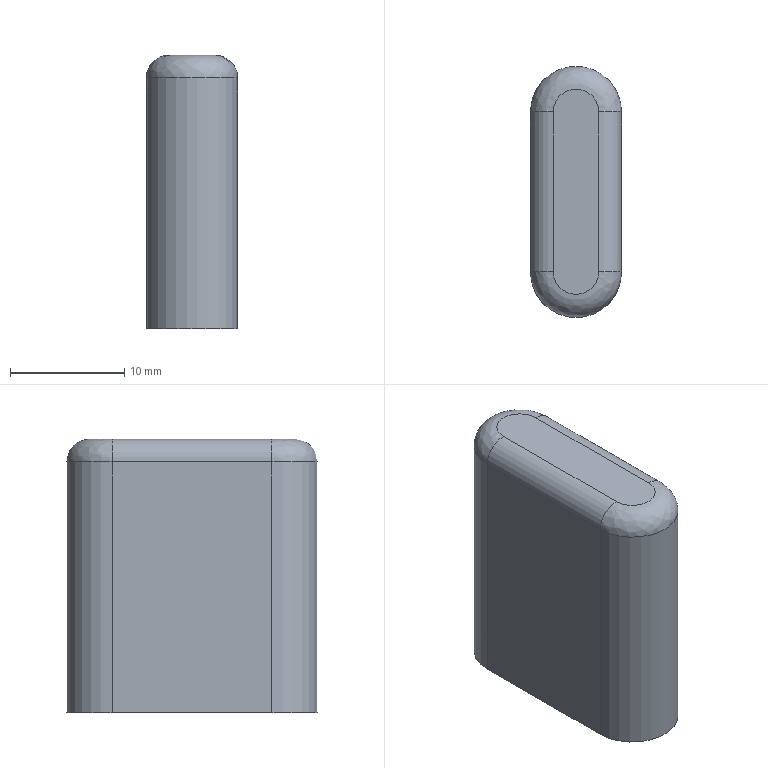Part | STEP file | Tube feed_id510_x_t | 1 solid | 10 faces | box 8 x 22 x 24 mm | volume 3851 mm3 | plane 4 | cylinder 4 | spline 2 | commonest cylinder face diameters 4 x2 8 x2
STEP:
#1=CARTESIAN_POINT('',(0.,0.,0.));
#2=DIRECTION('',(0.,0.,1.));
#3=DIRECTION('',(1.,0.,0.));
#4=AXIS2_PLACEMENT_3D('',#1,#2,#3);
#5=CARTESIAN_POINT('',(380.,467.436,-19.));
#6=VERTEX_POINT('',#5);
#7=CARTESIAN_POINT('',(380.,453.436,-19.));
#8=VERTEX_POINT('',#7);
#9=CARTESIAN_POINT('',(380.,449.436,-19.));
#10=DIRECTION('',(0.,-1.,0.));
#11=VECTOR('',#10,1.);
#12=LINE('',#9,#11);
#13=CARTESIAN_POINT('',(372.,449.436,-19.));
#14=DIRECTION('',(0.,0.,-1.));
#15=DIRECTION('',(0.,1.,0.));
#16=AXIS2_PLACEMENT_3D('',#13,#14,#15);
#17=PLANE('',#16);
#18=CARTESIAN_POINT('',(0.,8.));
#19=DIRECTION('',(-1.,0.));
#20=VECTOR('',#19,1.);
#21=LINE('',#18,#20);
#22=(GEOMETRIC_REPRESENTATION_CONTEXT(2)PARAMETRIC_REPRESENTATION_CONTEXT()REPRESENTATION_CONTEXT('',''));
#23=DEFINITIONAL_REPRESENTATION('',(#21),#22);
#24=PCURVE('',#17,#23);
#25=CARTESIAN_POINT('',(380.,449.436,-18.5));
#26=DIRECTION('',(-1.,0.,0.));
#27=DIRECTION('',(0.,0.,-1.));
#28=AXIS2_PLACEMENT_3D('',#25,#26,#27);
#29=PLANE('',#28);
#30=CARTESIAN_POINT('',(0.5,0.));
#31=DIRECTION('',(0.,1.));
#32=VECTOR('',#31,1.);
#33=LINE('',#30,#32);
#34=(GEOMETRIC_REPRESENTATION_CONTEXT(2)PARAMETRIC_REPRESENTATION_CONTEXT()REPRESENTATION_CONTEXT('',''));
#35=DEFINITIONAL_REPRESENTATION('',(#33),#34);
#36=PCURVE('',#29,#35);
#37=SURFACE_CURVE('',#12,(#24,#36),.PCURVE_S1.);
#38=EDGE_CURVE('',#6,#8,#37,.T.);
#39=ORIENTED_EDGE('',*,*,#38,.T.);
#40=CARTESIAN_POINT('',(372.,453.436,-19.));
#41=VERTEX_POINT('',#40);
#42=CARTESIAN_POINT('',(376.,453.436,-19.));
#43=DIRECTION('',(0.,0.,-1.));
#44=DIRECTION('',(0.,1.,0.));
#45=AXIS2_PLACEMENT_3D('',#42,#43,#44);
#46=CIRCLE('',#45,4.);
#47=CARTESIAN_POINT('',(4.,4.));
#48=DIRECTION('',(1.,0.));
#49=AXIS2_PLACEMENT_2D('',#47,#48);
#50=CIRCLE('',#49,4.);
#51=(GEOMETRIC_REPRESENTATION_CONTEXT(2)PARAMETRIC_REPRESENTATION_CONTEXT()REPRESENTATION_CONTEXT('',''));
#52=DEFINITIONAL_REPRESENTATION('',(#50),#51);
#53=PCURVE('',#17,#52);
#54=CARTESIAN_POINT('',(376.,453.436,-18.5));
#55=DIRECTION('',(0.,0.,-1.));
#56=DIRECTION('',(1.,0.,0.));
#57=AXIS2_PLACEMENT_3D('',#54,#55,#56);
#58=CYLINDRICAL_SURFACE('',#57,4.);
#59=CARTESIAN_POINT('',(-1.571,0.5));
#60=DIRECTION('',(1.,0.));
#61=VECTOR('',#60,1.);
#62=LINE('',#59,#61);
#63=(GEOMETRIC_REPRESENTATION_CONTEXT(2)PARAMETRIC_REPRESENTATION_CONTEXT()REPRESENTATION_CONTEXT('',''));
#64=DEFINITIONAL_REPRESENTATION('',(#62),#63);
#65=PCURVE('',#58,#64);
#66=SURFACE_CURVE('',#46,(#53,#65),.PCURVE_S1.);
#67=EDGE_CURVE('',#8,#41,#66,.T.);
#68=ORIENTED_EDGE('',*,*,#67,.T.);
#69=CARTESIAN_POINT('',(372.,467.436,-19.));
#70=VERTEX_POINT('',#69);
#71=CARTESIAN_POINT('',(372.,449.436,-19.));
#72=DIRECTION('',(0.,-1.,0.));
#73=VECTOR('',#72,1.);
#74=LINE('',#71,#73);
#75=CARTESIAN_POINT('',(0.,0.));
#76=DIRECTION('',(-1.,0.));
#77=VECTOR('',#76,1.);
#78=LINE('',#75,#77);
#79=(GEOMETRIC_REPRESENTATION_CONTEXT(2)PARAMETRIC_REPRESENTATION_CONTEXT()REPRESENTATION_CONTEXT('',''));
#80=DEFINITIONAL_REPRESENTATION('',(#78),#79);
#81=PCURVE('',#17,#80);
#82=CARTESIAN_POINT('',(372.,449.436,-18.5));
#83=DIRECTION('',(-1.,0.,0.));
#84=DIRECTION('',(0.,0.,-1.));
#85=AXIS2_PLACEMENT_3D('',#82,#83,#84);
#86=PLANE('',#85);
#87=CARTESIAN_POINT('',(0.5,0.));
#88=DIRECTION('',(0.,1.));
#89=VECTOR('',#88,1.);
#90=LINE('',#87,#89);
#91=(GEOMETRIC_REPRESENTATION_CONTEXT(2)PARAMETRIC_REPRESENTATION_CONTEXT()REPRESENTATION_CONTEXT('',''));
#92=DEFINITIONAL_REPRESENTATION('',(#90),#91);
#93=PCURVE('',#86,#92);
#94=SURFACE_CURVE('',#74,(#81,#93),.PCURVE_S1.);
#95=EDGE_CURVE('',#70,#41,#94,.T.);
#96=ORIENTED_EDGE('',*,*,#95,.F.);
#97=CARTESIAN_POINT('',(376.,467.436,-19.));
#98=DIRECTION('',(0.,0.,-1.));
#99=DIRECTION('',(0.,1.,0.));
#100=AXIS2_PLACEMENT_3D('',#97,#98,#99);
#101=CIRCLE('',#100,4.);
#102=CARTESIAN_POINT('',(18.,4.));
#103=DIRECTION('',(1.,0.));
#104=AXIS2_PLACEMENT_2D('',#102,#103);
#105=CIRCLE('',#104,4.);
#106=(GEOMETRIC_REPRESENTATION_CONTEXT(2)PARAMETRIC_REPRESENTATION_CONTEXT()REPRESENTATION_CONTEXT('',''));
#107=DEFINITIONAL_REPRESENTATION('',(#105),#106);
#108=PCURVE('',#17,#107);
#109=CARTESIAN_POINT('',(376.,467.436,-18.5));
#110=DIRECTION('',(0.,0.,1.));
#111=DIRECTION('',(-1.,0.,0.));
#112=AXIS2_PLACEMENT_3D('',#109,#110,#111);
#113=CYLINDRICAL_SURFACE('',#112,4.);
#114=CARTESIAN_POINT('',(10.996,-0.5));
#115=DIRECTION('',(-1.,0.));
#116=VECTOR('',#115,1.);
#117=LINE('',#114,#116);
#118=(GEOMETRIC_REPRESENTATION_CONTEXT(2)PARAMETRIC_REPRESENTATION_CONTEXT()REPRESENTATION_CONTEXT('',''));
#119=DEFINITIONAL_REPRESENTATION('',(#117),#118);
#120=PCURVE('',#113,#119);
#121=SURFACE_CURVE('',#101,(#108,#120),.PCURVE_S1.);
#122=EDGE_CURVE('',#70,#6,#121,.T.);
#123=ORIENTED_EDGE('',*,*,#122,.T.);
#124=EDGE_LOOP('',(#39,#68,#96,#123));
#125=FACE_BOUND('',#124,.T.);
#126=ADVANCED_FACE('',(#125),#17,.T.);
#127=CARTESIAN_POINT('',(378.,467.436,5.));
#128=VERTEX_POINT('',#127);
#129=CARTESIAN_POINT('',(374.,467.436,5.));
#130=VERTEX_POINT('',#129);
#131=CARTESIAN_POINT('',(376.,467.436,5.));
#132=DIRECTION('',(0.,0.,1.));
#133=DIRECTION('',(0.,1.,0.));
#134=AXIS2_PLACEMENT_3D('',#131,#132,#133);
#135=CIRCLE('',#134,2.);
#136=CARTESIAN_POINT('',(372.,449.436,5.));
#137=DIRECTION('',(0.,0.,-1.));
#138=DIRECTION('',(0.,1.,0.));
#139=AXIS2_PLACEMENT_3D('',#136,#137,#138);
#140=PLANE('',#139);
#141=CARTESIAN_POINT('',(20.,4.));
#142=CARTESIAN_POINT('',(20.,0.5359));
#143=CARTESIAN_POINT('',(17.,2.268));
#144=CARTESIAN_POINT('',(14.,4.));
#145=CARTESIAN_POINT('',(17.,5.732));
#146=CARTESIAN_POINT('',(20.,7.464));
#147=CARTESIAN_POINT('',(20.,4.));
#148=(BOUNDED_CURVE()B_SPLINE_CURVE(2,(#141,#142,#143,#144,#145,#146,#147),.UNSPECIFIED.,.T.,.F.)B_SPLINE_CURVE_WITH_KNOTS((1,2,2,2,2,1),(-2.094,0.,2.094,4.189,6.283,8.378),.UNSPECIFIED.)CURVE()GEOMETRIC_REPRESENTATION_ITEM()RATIONAL_B_SPLINE_CURVE((1.,0.5,1.,0.5,1.,0.5,1.))REPRESENTATION_ITEM(''));
#149=(GEOMETRIC_REPRESENTATION_CONTEXT(2)PARAMETRIC_REPRESENTATION_CONTEXT()REPRESENTATION_CONTEXT('',''));
#150=DEFINITIONAL_REPRESENTATION('',(#148),#149);
#151=PCURVE('',#140,#150);
#152=CARTESIAN_POINT('',(372.,467.436,3.));
#153=CARTESIAN_POINT('',(372.,475.436,3.));
#154=CARTESIAN_POINT('',(380.,475.436,3.));
#155=CARTESIAN_POINT('',(380.,467.436,3.));
#156=CARTESIAN_POINT('',(372.,467.436,4.172));
#157=CARTESIAN_POINT('',(372.,475.436,4.172));
#158=CARTESIAN_POINT('',(380.,475.436,4.172));
#159=CARTESIAN_POINT('',(380.,467.436,4.172));
#160=CARTESIAN_POINT('',(372.828,467.436,5.));
#161=CARTESIAN_POINT('',(372.828,473.779,5.));
#162=CARTESIAN_POINT('',(379.172,473.779,5.));
#163=CARTESIAN_POINT('',(379.172,467.436,5.));
#164=CARTESIAN_POINT('',(374.,467.436,5.));
#165=CARTESIAN_POINT('',(374.,471.436,5.));
#166=CARTESIAN_POINT('',(378.,471.436,5.));
#167=CARTESIAN_POINT('',(378.,467.436,5.));
#168=(BOUNDED_SURFACE()B_SPLINE_SURFACE(3,3,((#152,#153,#154,#155),(#156,#157,#158,#159),(#160,#161,#162,#163),(#164,#165,#166,#167)),.UNSPECIFIED.,.F.,.F.,.F.)B_SPLINE_SURFACE_WITH_KNOTS((4,4),(4,4),(0.,1.),(0.,1.),.PIECEWISE_BEZIER_KNOTS.)GEOMETRIC_REPRESENTATION_ITEM()RATIONAL_B_SPLINE_SURFACE(((1.,0.3333,0.3333,1.),(0.8047,0.2682,0.2682,0.8047),(0.8047,0.2682,0.2682,0.8047),(1.,0.3333,0.3333,1.)))REPRESENTATION_ITEM('')SURFACE());
#169=CARTESIAN_POINT('',(1.,1.));
#170=CARTESIAN_POINT('',(1.,0.9763));
#171=CARTESIAN_POINT('',(1.,0.9319));
#172=CARTESIAN_POINT('',(1.,0.8733));
#173=CARTESIAN_POINT('',(1.,0.8206));
#174=CARTESIAN_POINT('',(1.,0.7724));
#175=CARTESIAN_POINT('',(1.,0.7279));
#176=CARTESIAN_POINT('',(1.,0.6861));
#177=CARTESIAN_POINT('',(1.,0.6465));
#178=CARTESIAN_POINT('',(1.,0.6086));
#179=CARTESIAN_POINT('',(1.,0.5718));
#180=CARTESIAN_POINT('',(1.,0.5357));
#181=CARTESIAN_POINT('',(1.,0.5));
#182=CARTESIAN_POINT('',(1.,0.4643));
#183=CARTESIAN_POINT('',(1.,0.4282));
#184=CARTESIAN_POINT('',(1.,0.3914));
#185=CARTESIAN_POINT('',(1.,0.3535));
#186=CARTESIAN_POINT('',(1.,0.3139));
#187=CARTESIAN_POINT('',(1.,0.2721));
#188=CARTESIAN_POINT('',(1.,0.2276));
#189=CARTESIAN_POINT('',(1.,0.1794));
#190=CARTESIAN_POINT('',(1.,0.1267));
#191=CARTESIAN_POINT('',(1.,0.06805));
#192=CARTESIAN_POINT('',(1.,0.02375));
#193=CARTESIAN_POINT('',(1.,0.));
#194=B_SPLINE_CURVE_WITH_KNOTS('',3,(#169,#170,#171,#172,#173,#174,#175,#176,#177,#178,#179,#180,#181,#182,#183,#184,#185,#186,#187,#188,#189,#190,#191,#192,#193),.UNSPECIFIED.,.F.,.F.,(4,1,1,1,1,1,1,1,1,1,1,1,1,1,1,1,1,1,1,1,1,1,4),(4.712,4.855,4.998,5.141,5.284,5.426,5.569,5.712,5.855,5.998,6.14,6.283,6.426,6.569,6.712,6.854,6.997,7.14,7.283,7.426,7.568,7.711,7.854),.QUASI_UNIFORM_KNOTS.);
#195=(GEOMETRIC_REPRESENTATION_CONTEXT(2)PARAMETRIC_REPRESENTATION_CONTEXT()REPRESENTATION_CONTEXT('',''));
#196=DEFINITIONAL_REPRESENTATION('',(#194),#195);
#197=PCURVE('',#168,#196);
#198=SURFACE_CURVE('',#135,(#151,#197),.PCURVE_S1.);
#199=EDGE_CURVE('',#128,#130,#198,.T.);
#200=ORIENTED_EDGE('',*,*,#199,.T.);
#201=CARTESIAN_POINT('',(374.,453.436,5.));
#202=VERTEX_POINT('',#201);
#203=CARTESIAN_POINT('',(374.,449.436,5.));
#204=DIRECTION('',(0.,-1.,0.));
#205=VECTOR('',#204,1.);
#206=LINE('',#203,#205);
#207=CARTESIAN_POINT('',(0.,2.));
#208=DIRECTION('',(-1.,0.));
#209=VECTOR('',#208,1.);
#210=LINE('',#207,#209);
#211=(GEOMETRIC_REPRESENTATION_CONTEXT(2)PARAMETRIC_REPRESENTATION_CONTEXT()REPRESENTATION_CONTEXT('',''));
#212=DEFINITIONAL_REPRESENTATION('',(#210),#211);
#213=PCURVE('',#140,#212);
#214=CARTESIAN_POINT('',(374.,449.436,3.));
#215=DIRECTION('',(0.,1.,0.));
#216=DIRECTION('',(0.,0.,1.));
#217=AXIS2_PLACEMENT_3D('',#214,#215,#216);
#218=CYLINDRICAL_SURFACE('',#217,2.);
#219=CARTESIAN_POINT('',(6.283,0.));
#220=DIRECTION('',(0.,-1.));
#221=VECTOR('',#220,1.);
#222=LINE('',#219,#221);
#223=(GEOMETRIC_REPRESENTATION_CONTEXT(2)PARAMETRIC_REPRESENTATION_CONTEXT()REPRESENTATION_CONTEXT('',''));
#224=DEFINITIONAL_REPRESENTATION('',(#222),#223);
#225=PCURVE('',#218,#224);
#226=SURFACE_CURVE('',#206,(#213,#225),.PCURVE_S1.);
#227=EDGE_CURVE('',#130,#202,#226,.T.);
#228=ORIENTED_EDGE('',*,*,#227,.T.);
#229=CARTESIAN_POINT('',(378.,453.436,5.));
#230=VERTEX_POINT('',#229);
#231=CARTESIAN_POINT('',(376.,453.436,5.));
#232=DIRECTION('',(0.,0.,1.));
#233=DIRECTION('',(0.,1.,0.));
#234=AXIS2_PLACEMENT_3D('',#231,#232,#233);
#235=CIRCLE('',#234,2.);
#236=CARTESIAN_POINT('',(6.,4.));
#237=CARTESIAN_POINT('',(6.,0.5359));
#238=CARTESIAN_POINT('',(3.,2.268));
#239=CARTESIAN_POINT('',(0.,4.));
#240=CARTESIAN_POINT('',(3.,5.732));
#241=CARTESIAN_POINT('',(6.,7.464));
#242=CARTESIAN_POINT('',(6.,4.));
#243=(BOUNDED_CURVE()B_SPLINE_CURVE(2,(#236,#237,#238,#239,#240,#241,#242),.UNSPECIFIED.,.T.,.F.)B_SPLINE_CURVE_WITH_KNOTS((1,2,2,2,2,1),(-2.094,0.,2.094,4.189,6.283,8.378),.UNSPECIFIED.)CURVE()GEOMETRIC_REPRESENTATION_ITEM()RATIONAL_B_SPLINE_CURVE((1.,0.5,1.,0.5,1.,0.5,1.))REPRESENTATION_ITEM(''));
#244=(GEOMETRIC_REPRESENTATION_CONTEXT(2)PARAMETRIC_REPRESENTATION_CONTEXT()REPRESENTATION_CONTEXT('',''));
#245=DEFINITIONAL_REPRESENTATION('',(#243),#244);
#246=PCURVE('',#140,#245);
#247=CARTESIAN_POINT('',(380.,453.436,3.));
#248=CARTESIAN_POINT('',(380.,445.436,3.));
#249=CARTESIAN_POINT('',(372.,445.436,3.));
#250=CARTESIAN_POINT('',(372.,453.436,3.));
#251=CARTESIAN_POINT('',(380.,453.436,4.172));
#252=CARTESIAN_POINT('',(380.,445.436,4.172));
#253=CARTESIAN_POINT('',(372.,445.436,4.172));
#254=CARTESIAN_POINT('',(372.,453.436,4.172));
#255=CARTESIAN_POINT('',(379.172,453.436,5.));
#256=CARTESIAN_POINT('',(379.172,447.092,5.));
#257=CARTESIAN_POINT('',(372.828,447.092,5.));
#258=CARTESIAN_POINT('',(372.828,453.436,5.));
#259=CARTESIAN_POINT('',(378.,453.436,5.));
#260=CARTESIAN_POINT('',(378.,449.436,5.));
#261=CARTESIAN_POINT('',(374.,449.436,5.));
#262=CARTESIAN_POINT('',(374.,453.436,5.));
#263=(BOUNDED_SURFACE()B_SPLINE_SURFACE(3,3,((#247,#248,#249,#250),(#251,#252,#253,#254),(#255,#256,#257,#258),(#259,#260,#261,#262)),.UNSPECIFIED.,.F.,.F.,.F.)B_SPLINE_SURFACE_WITH_KNOTS((4,4),(4,4),(0.,1.),(0.,1.),.PIECEWISE_BEZIER_KNOTS.)GEOMETRIC_REPRESENTATION_ITEM()RATIONAL_B_SPLINE_SURFACE(((1.,0.3333,0.3333,1.),(0.8047,0.2682,0.2682,0.8047),(0.8047,0.2682,0.2682,0.8047),(1.,0.3333,0.3333,1.)))REPRESENTATION_ITEM('')SURFACE());
#264=CARTESIAN_POINT('',(1.,1.));
#265=CARTESIAN_POINT('',(1.,0.9763));
#266=CARTESIAN_POINT('',(1.,0.9319));
#267=CARTESIAN_POINT('',(1.,0.8733));
#268=CARTESIAN_POINT('',(1.,0.8206));
#269=CARTESIAN_POINT('',(1.,0.7724));
#270=CARTESIAN_POINT('',(1.,0.7279));
#271=CARTESIAN_POINT('',(1.,0.6861));
#272=CARTESIAN_POINT('',(1.,0.6465));
#273=CARTESIAN_POINT('',(1.,0.6086));
#274=CARTESIAN_POINT('',(1.,0.5718));
#275=CARTESIAN_POINT('',(1.,0.5357));
#276=CARTESIAN_POINT('',(1.,0.5));
#277=CARTESIAN_POINT('',(1.,0.4643));
#278=CARTESIAN_POINT('',(1.,0.4282));
#279=CARTESIAN_POINT('',(1.,0.3914));
#280=CARTESIAN_POINT('',(1.,0.3535));
#281=CARTESIAN_POINT('',(1.,0.3139));
#282=CARTESIAN_POINT('',(1.,0.2721));
#283=CARTESIAN_POINT('',(1.,0.2276));
#284=CARTESIAN_POINT('',(1.,0.1794));
#285=CARTESIAN_POINT('',(1.,0.1267));
#286=CARTESIAN_POINT('',(1.,0.06805));
#287=CARTESIAN_POINT('',(1.,0.02375));
#288=CARTESIAN_POINT('',(1.,0.));
#289=B_SPLINE_CURVE_WITH_KNOTS('',3,(#264,#265,#266,#267,#268,#269,#270,#271,#272,#273,#274,#275,#276,#277,#278,#279,#280,#281,#282,#283,#284,#285,#286,#287,#288),.UNSPECIFIED.,.F.,.F.,(4,1,1,1,1,1,1,1,1,1,1,1,1,1,1,1,1,1,1,1,1,1,4),(1.571,1.714,1.856,1.999,2.142,2.285,2.428,2.57,2.713,2.856,2.999,3.142,3.284,3.427,3.57,3.713,3.856,3.998,4.141,4.284,4.427,4.57,4.712),.QUASI_UNIFORM_KNOTS.);
#290=(GEOMETRIC_REPRESENTATION_CONTEXT(2)PARAMETRIC_REPRESENTATION_CONTEXT()REPRESENTATION_CONTEXT('',''));
#291=DEFINITIONAL_REPRESENTATION('',(#289),#290);
#292=PCURVE('',#263,#291);
#293=SURFACE_CURVE('',#235,(#246,#292),.PCURVE_S1.);
#294=EDGE_CURVE('',#202,#230,#293,.T.);
#295=ORIENTED_EDGE('',*,*,#294,.T.);
#296=CARTESIAN_POINT('',(378.,453.436,5.));
#297=DIRECTION('',(0.,1.,0.));
#298=VECTOR('',#297,1.);
#299=LINE('',#296,#298);
#300=CARTESIAN_POINT('',(4.,6.));
#301=DIRECTION('',(1.,0.));
#302=VECTOR('',#301,1.);
#303=LINE('',#300,#302);
#304=(GEOMETRIC_REPRESENTATION_CONTEXT(2)PARAMETRIC_REPRESENTATION_CONTEXT()REPRESENTATION_CONTEXT('',''));
#305=DEFINITIONAL_REPRESENTATION('',(#303),#304);
#306=PCURVE('',#140,#305);
#307=CARTESIAN_POINT('',(378.,449.436,3.));
#308=DIRECTION('',(0.,-1.,0.));
#309=DIRECTION('',(0.,0.,-1.));
#310=AXIS2_PLACEMENT_3D('',#307,#308,#309);
#311=CYLINDRICAL_SURFACE('',#310,2.);
#312=CARTESIAN_POINT('',(3.142,-4.));
#313=DIRECTION('',(0.,-1.));
#314=VECTOR('',#313,1.);
#315=LINE('',#312,#314);
#316=(GEOMETRIC_REPRESENTATION_CONTEXT(2)PARAMETRIC_REPRESENTATION_CONTEXT()REPRESENTATION_CONTEXT('',''));
#317=DEFINITIONAL_REPRESENTATION('',(#315),#316);
#318=PCURVE('',#311,#317);
#319=SURFACE_CURVE('',#299,(#306,#318),.PCURVE_S1.);
#320=EDGE_CURVE('',#230,#128,#319,.T.);
#321=ORIENTED_EDGE('',*,*,#320,.T.);
#322=EDGE_LOOP('',(#200,#228,#295,#321));
#323=FACE_BOUND('',#322,.T.);
#324=ADVANCED_FACE('',(#323),#140,.F.);
#325=CARTESIAN_POINT('',(380.,453.436,3.));
#326=VERTEX_POINT('',#325);
#327=CARTESIAN_POINT('',(380.,453.436,5.));
#328=DIRECTION('',(0.,0.,-1.));
#329=VECTOR('',#328,1.);
#330=LINE('',#327,#329);
#331=CARTESIAN_POINT('',(-23.5,-4.));
#332=DIRECTION('',(1.,0.));
#333=VECTOR('',#332,1.);
#334=LINE('',#331,#333);
#335=(GEOMETRIC_REPRESENTATION_CONTEXT(2)PARAMETRIC_REPRESENTATION_CONTEXT()REPRESENTATION_CONTEXT('',''));
#336=DEFINITIONAL_REPRESENTATION('',(#334),#335);
#337=PCURVE('',#29,#336);
#338=CARTESIAN_POINT('',(0.,-23.5));
#339=DIRECTION('',(0.,1.));
#340=VECTOR('',#339,1.);
#341=LINE('',#338,#340);
#342=(GEOMETRIC_REPRESENTATION_CONTEXT(2)PARAMETRIC_REPRESENTATION_CONTEXT()REPRESENTATION_CONTEXT('',''));
#343=DEFINITIONAL_REPRESENTATION('',(#341),#342);
#344=PCURVE('',#58,#343);
#345=SURFACE_CURVE('',#330,(#337,#344),.PCURVE_S1.);
#346=EDGE_CURVE('',#326,#8,#345,.T.);
#347=ORIENTED_EDGE('',*,*,#346,.T.);
#348=ORIENTED_EDGE('',*,*,#38,.F.);
#349=CARTESIAN_POINT('',(380.,467.436,3.));
#350=VERTEX_POINT('',#349);
#351=CARTESIAN_POINT('',(380.,467.436,-18.5));
#352=DIRECTION('',(0.,0.,1.));
#353=VECTOR('',#352,1.);
#354=LINE('',#351,#353);
#355=CARTESIAN_POINT('',(0.,-18.));
#356=DIRECTION('',(-1.,0.));
#357=VECTOR('',#356,1.);
#358=LINE('',#355,#357);
#359=(GEOMETRIC_REPRESENTATION_CONTEXT(2)PARAMETRIC_REPRESENTATION_CONTEXT()REPRESENTATION_CONTEXT('',''));
#360=DEFINITIONAL_REPRESENTATION('',(#358),#359);
#361=PCURVE('',#29,#360);
#362=CARTESIAN_POINT('',(3.142,0.));
#363=DIRECTION('',(0.,1.));
#364=VECTOR('',#363,1.);
#365=LINE('',#362,#364);
#366=(GEOMETRIC_REPRESENTATION_CONTEXT(2)PARAMETRIC_REPRESENTATION_CONTEXT()REPRESENTATION_CONTEXT('',''));
#367=DEFINITIONAL_REPRESENTATION('',(#365),#366);
#368=PCURVE('',#113,#367);
#369=SURFACE_CURVE('',#354,(#361,#368),.PCURVE_S1.);
#370=EDGE_CURVE('',#6,#350,#369,.T.);
#371=ORIENTED_EDGE('',*,*,#370,.T.);
#372=CARTESIAN_POINT('',(380.,467.436,3.));
#373=DIRECTION('',(0.,-1.,0.));
#374=VECTOR('',#373,1.);
#375=LINE('',#372,#374);
#376=CARTESIAN_POINT('',(-21.5,-18.));
#377=DIRECTION('',(0.,1.));
#378=VECTOR('',#377,1.);
#379=LINE('',#376,#378);
#380=(GEOMETRIC_REPRESENTATION_CONTEXT(2)PARAMETRIC_REPRESENTATION_CONTEXT()REPRESENTATION_CONTEXT('',''));
#381=DEFINITIONAL_REPRESENTATION('',(#379),#380);
#382=PCURVE('',#29,#381);
#383=CARTESIAN_POINT('',(1.571,-18.));
#384=DIRECTION('',(0.,1.));
#385=VECTOR('',#384,1.);
#386=LINE('',#383,#385);
#387=(GEOMETRIC_REPRESENTATION_CONTEXT(2)PARAMETRIC_REPRESENTATION_CONTEXT()REPRESENTATION_CONTEXT('',''));
#388=DEFINITIONAL_REPRESENTATION('',(#386),#387);
#389=PCURVE('',#311,#388);
#390=SURFACE_CURVE('',#375,(#382,#389),.PCURVE_S1.);
#391=EDGE_CURVE('',#350,#326,#390,.T.);
#392=ORIENTED_EDGE('',*,*,#391,.T.);
#393=EDGE_LOOP('',(#347,#348,#371,#392));
#394=FACE_BOUND('',#393,.T.);
#395=ADVANCED_FACE('',(#394),#29,.F.);
#396=CARTESIAN_POINT('',(372.,467.436,3.));
#397=VERTEX_POINT('',#396);
#398=CARTESIAN_POINT('',(372.,467.436,-18.5));
#399=DIRECTION('',(0.,0.,-1.));
#400=VECTOR('',#399,1.);
#401=LINE('',#398,#400);
#402=CARTESIAN_POINT('',(0.,-18.));
#403=DIRECTION('',(1.,0.));
#404=VECTOR('',#403,1.);
#405=LINE('',#402,#404);
#406=(GEOMETRIC_REPRESENTATION_CONTEXT(2)PARAMETRIC_REPRESENTATION_CONTEXT()REPRESENTATION_CONTEXT('',''));
#407=DEFINITIONAL_REPRESENTATION('',(#405),#406);
#408=PCURVE('',#86,#407);
#409=CARTESIAN_POINT('',(6.283,0.));
#410=DIRECTION('',(0.,-1.));
#411=VECTOR('',#410,1.);
#412=LINE('',#409,#411);
#413=(GEOMETRIC_REPRESENTATION_CONTEXT(2)PARAMETRIC_REPRESENTATION_CONTEXT()REPRESENTATION_CONTEXT('',''));
#414=DEFINITIONAL_REPRESENTATION('',(#412),#413);
#415=PCURVE('',#113,#414);
#416=SURFACE_CURVE('',#401,(#408,#415),.PCURVE_S1.);
#417=EDGE_CURVE('',#397,#70,#416,.T.);
#418=ORIENTED_EDGE('',*,*,#417,.T.);
#419=ORIENTED_EDGE('',*,*,#95,.T.);
#420=CARTESIAN_POINT('',(372.,453.436,3.));
#421=VERTEX_POINT('',#420);
#422=CARTESIAN_POINT('',(372.,453.436,-18.5));
#423=DIRECTION('',(0.,0.,1.));
#424=VECTOR('',#423,1.);
#425=LINE('',#422,#424);
#426=CARTESIAN_POINT('',(0.,-4.));
#427=DIRECTION('',(-1.,0.));
#428=VECTOR('',#427,1.);
#429=LINE('',#426,#428);
#430=(GEOMETRIC_REPRESENTATION_CONTEXT(2)PARAMETRIC_REPRESENTATION_CONTEXT()REPRESENTATION_CONTEXT('',''));
#431=DEFINITIONAL_REPRESENTATION('',(#429),#430);
#432=PCURVE('',#86,#431);
#433=CARTESIAN_POINT('',(3.142,0.));
#434=DIRECTION('',(0.,-1.));
#435=VECTOR('',#434,1.);
#436=LINE('',#433,#435);
#437=(GEOMETRIC_REPRESENTATION_CONTEXT(2)PARAMETRIC_REPRESENTATION_CONTEXT()REPRESENTATION_CONTEXT('',''));
#438=DEFINITIONAL_REPRESENTATION('',(#436),#437);
#439=PCURVE('',#58,#438);
#440=SURFACE_CURVE('',#425,(#432,#439),.PCURVE_S1.);
#441=EDGE_CURVE('',#41,#421,#440,.T.);
#442=ORIENTED_EDGE('',*,*,#441,.T.);
#443=CARTESIAN_POINT('',(372.,449.436,3.));
#444=DIRECTION('',(0.,1.,0.));
#445=VECTOR('',#444,1.);
#446=LINE('',#443,#445);
#447=CARTESIAN_POINT('',(-21.5,0.));
#448=DIRECTION('',(0.,-1.));
#449=VECTOR('',#448,1.);
#450=LINE('',#447,#449);
#451=(GEOMETRIC_REPRESENTATION_CONTEXT(2)PARAMETRIC_REPRESENTATION_CONTEXT()REPRESENTATION_CONTEXT('',''));
#452=DEFINITIONAL_REPRESENTATION('',(#450),#451);
#453=PCURVE('',#86,#452);
#454=CARTESIAN_POINT('',(4.712,0.));
#455=DIRECTION('',(0.,1.));
#456=VECTOR('',#455,1.);
#457=LINE('',#454,#456);
#458=(GEOMETRIC_REPRESENTATION_CONTEXT(2)PARAMETRIC_REPRESENTATION_CONTEXT()REPRESENTATION_CONTEXT('',''));
#459=DEFINITIONAL_REPRESENTATION('',(#457),#458);
#460=PCURVE('',#218,#459);
#461=SURFACE_CURVE('',#446,(#453,#460),.PCURVE_S1.);
#462=EDGE_CURVE('',#421,#397,#461,.T.);
#463=ORIENTED_EDGE('',*,*,#462,.T.);
#464=EDGE_LOOP('',(#418,#419,#442,#463));
#465=FACE_BOUND('',#464,.T.);
#466=ADVANCED_FACE('',(#465),#86,.T.);
#467=ORIENTED_EDGE('',*,*,#370,.F.);
#468=ORIENTED_EDGE('',*,*,#122,.F.);
#469=ORIENTED_EDGE('',*,*,#417,.F.);
#470=CARTESIAN_POINT('',(376.,467.436,3.));
#471=DIRECTION('',(0.,0.,-1.));
#472=DIRECTION('',(0.,1.,0.));
#473=AXIS2_PLACEMENT_3D('',#470,#471,#472);
#474=CIRCLE('',#473,4.);
#475=CARTESIAN_POINT('',(10.996,21.5));
#476=DIRECTION('',(-1.,0.));
#477=VECTOR('',#476,1.);
#478=LINE('',#475,#477);
#479=(GEOMETRIC_REPRESENTATION_CONTEXT(2)PARAMETRIC_REPRESENTATION_CONTEXT()REPRESENTATION_CONTEXT('',''));
#480=DEFINITIONAL_REPRESENTATION('',(#478),#479);
#481=PCURVE('',#113,#480);
#482=CARTESIAN_POINT('',(0.,0.));
#483=CARTESIAN_POINT('',(0.,0.02375));
#484=CARTESIAN_POINT('',(0.,0.06805));
#485=CARTESIAN_POINT('',(0.,0.1267));
#486=CARTESIAN_POINT('',(0.,0.1794));
#487=CARTESIAN_POINT('',(0.,0.2276));
#488=CARTESIAN_POINT('',(0.,0.2721));
#489=CARTESIAN_POINT('',(0.,0.3139));
#490=CARTESIAN_POINT('',(0.,0.3535));
#491=CARTESIAN_POINT('',(0.,0.3914));
#492=CARTESIAN_POINT('',(0.,0.4282));
#493=CARTESIAN_POINT('',(0.,0.4643));
#494=CARTESIAN_POINT('',(0.,0.5));
#495=CARTESIAN_POINT('',(0.,0.5357));
#496=CARTESIAN_POINT('',(0.,0.5718));
#497=CARTESIAN_POINT('',(0.,0.6086));
#498=CARTESIAN_POINT('',(0.,0.6465));
#499=CARTESIAN_POINT('',(0.,0.6861));
#500=CARTESIAN_POINT('',(0.,0.7279));
#501=CARTESIAN_POINT('',(0.,0.7724));
#502=CARTESIAN_POINT('',(0.,0.8206));
#503=CARTESIAN_POINT('',(0.,0.8733));
#504=CARTESIAN_POINT('',(0.,0.9319));
#505=CARTESIAN_POINT('',(0.,0.9763));
#506=CARTESIAN_POINT('',(0.,1.));
#507=B_SPLINE_CURVE_WITH_KNOTS('',3,(#482,#483,#484,#485,#486,#487,#488,#489,#490,#491,#492,#493,#494,#495,#496,#497,#498,#499,#500,#501,#502,#503,#504,#505,#506),.UNSPECIFIED.,.F.,.F.,(4,1,1,1,1,1,1,1,1,1,1,1,1,1,1,1,1,1,1,1,1,1,4),(4.712,4.855,4.998,5.141,5.284,5.426,5.569,5.712,5.855,5.998,6.14,6.283,6.426,6.569,6.712,6.854,6.997,7.14,7.283,7.426,7.568,7.711,7.854),.QUASI_UNIFORM_KNOTS.);
#508=(GEOMETRIC_REPRESENTATION_CONTEXT(2)PARAMETRIC_REPRESENTATION_CONTEXT()REPRESENTATION_CONTEXT('',''));
#509=DEFINITIONAL_REPRESENTATION('',(#507),#508);
#510=PCURVE('',#168,#509);
#511=SURFACE_CURVE('',#474,(#481,#510),.PCURVE_S1.);
#512=EDGE_CURVE('',#397,#350,#511,.T.);
#513=ORIENTED_EDGE('',*,*,#512,.T.);
#514=EDGE_LOOP('',(#467,#468,#469,#513));
#515=FACE_BOUND('',#514,.T.);
#516=ADVANCED_FACE('',(#515),#113,.T.);
#517=ORIENTED_EDGE('',*,*,#441,.F.);
#518=ORIENTED_EDGE('',*,*,#67,.F.);
#519=ORIENTED_EDGE('',*,*,#346,.F.);
#520=CARTESIAN_POINT('',(376.,453.436,3.));
#521=DIRECTION('',(0.,0.,-1.));
#522=DIRECTION('',(0.,1.,0.));
#523=AXIS2_PLACEMENT_3D('',#520,#521,#522);
#524=CIRCLE('',#523,4.);
#525=CARTESIAN_POINT('',(-1.571,-21.5));
#526=DIRECTION('',(1.,0.));
#527=VECTOR('',#526,1.);
#528=LINE('',#525,#527);
#529=(GEOMETRIC_REPRESENTATION_CONTEXT(2)PARAMETRIC_REPRESENTATION_CONTEXT()REPRESENTATION_CONTEXT('',''));
#530=DEFINITIONAL_REPRESENTATION('',(#528),#529);
#531=PCURVE('',#58,#530);
#532=CARTESIAN_POINT('',(0.,0.));
#533=CARTESIAN_POINT('',(0.,0.02375));
#534=CARTESIAN_POINT('',(0.,0.06805));
#535=CARTESIAN_POINT('',(0.,0.1267));
#536=CARTESIAN_POINT('',(0.,0.1794));
#537=CARTESIAN_POINT('',(0.,0.2276));
#538=CARTESIAN_POINT('',(0.,0.2721));
#539=CARTESIAN_POINT('',(0.,0.3139));
#540=CARTESIAN_POINT('',(0.,0.3535));
#541=CARTESIAN_POINT('',(0.,0.3914));
#542=CARTESIAN_POINT('',(0.,0.4282));
#543=CARTESIAN_POINT('',(0.,0.4643));
#544=CARTESIAN_POINT('',(0.,0.5));
#545=CARTESIAN_POINT('',(0.,0.5357));
#546=CARTESIAN_POINT('',(0.,0.5718));
#547=CARTESIAN_POINT('',(0.,0.6086));
#548=CARTESIAN_POINT('',(0.,0.6465));
#549=CARTESIAN_POINT('',(0.,0.6861));
#550=CARTESIAN_POINT('',(0.,0.7279));
#551=CARTESIAN_POINT('',(0.,0.7724));
#552=CARTESIAN_POINT('',(0.,0.8206));
#553=CARTESIAN_POINT('',(0.,0.8733));
#554=CARTESIAN_POINT('',(0.,0.9319));
#555=CARTESIAN_POINT('',(0.,0.9763));
#556=CARTESIAN_POINT('',(0.,1.));
#557=B_SPLINE_CURVE_WITH_KNOTS('',3,(#532,#533,#534,#535,#536,#537,#538,#539,#540,#541,#542,#543,#544,#545,#546,#547,#548,#549,#550,#551,#552,#553,#554,#555,#556),.UNSPECIFIED.,.F.,.F.,(4,1,1,1,1,1,1,1,1,1,1,1,1,1,1,1,1,1,1,1,1,1,4),(1.571,1.714,1.856,1.999,2.142,2.285,2.428,2.57,2.713,2.856,2.999,3.142,3.284,3.427,3.57,3.713,3.856,3.998,4.141,4.284,4.427,4.57,4.712),.QUASI_UNIFORM_KNOTS.);
#558=(GEOMETRIC_REPRESENTATION_CONTEXT(2)PARAMETRIC_REPRESENTATION_CONTEXT()REPRESENTATION_CONTEXT('',''));
#559=DEFINITIONAL_REPRESENTATION('',(#557),#558);
#560=PCURVE('',#263,#559);
#561=SURFACE_CURVE('',#524,(#531,#560),.PCURVE_S1.);
#562=EDGE_CURVE('',#326,#421,#561,.T.);
#563=ORIENTED_EDGE('',*,*,#562,.T.);
#564=EDGE_LOOP('',(#517,#518,#519,#563));
#565=FACE_BOUND('',#564,.T.);
#566=ADVANCED_FACE('',(#565),#58,.T.);
#567=CARTESIAN_POINT('',(374.,453.436,3.));
#568=DIRECTION('',(0.,-1.,0.));
#569=DIRECTION('',(0.,0.,-1.));
#570=AXIS2_PLACEMENT_3D('',#567,#568,#569);
#571=CIRCLE('',#570,2.);
#572=CARTESIAN_POINT('',(9.425,4.));
#573=DIRECTION('',(-1.,0.));
#574=VECTOR('',#573,1.);
#575=LINE('',#572,#574);
#576=(GEOMETRIC_REPRESENTATION_CONTEXT(2)PARAMETRIC_REPRESENTATION_CONTEXT()REPRESENTATION_CONTEXT('',''));
#577=DEFINITIONAL_REPRESENTATION('',(#575),#576);
#578=PCURVE('',#218,#577);
#579=CARTESIAN_POINT('',(1.,1.));
#580=CARTESIAN_POINT('',(0.9832,1.));
#581=CARTESIAN_POINT('',(0.95,1.));
#582=CARTESIAN_POINT('',(0.9016,1.));
#583=CARTESIAN_POINT('',(0.8543,1.));
#584=CARTESIAN_POINT('',(0.808,1.));
#585=CARTESIAN_POINT('',(0.7625,1.));
#586=CARTESIAN_POINT('',(0.7177,1.));
#587=CARTESIAN_POINT('',(0.6735,1.));
#588=CARTESIAN_POINT('',(0.6297,1.));
#589=CARTESIAN_POINT('',(0.5863,1.));
#590=CARTESIAN_POINT('',(0.5431,1.));
#591=CARTESIAN_POINT('',(0.5,1.));
#592=CARTESIAN_POINT('',(0.4569,1.));
#593=CARTESIAN_POINT('',(0.4137,1.));
#594=CARTESIAN_POINT('',(0.3703,1.));
#595=CARTESIAN_POINT('',(0.3265,1.));
#596=CARTESIAN_POINT('',(0.2823,1.));
#597=CARTESIAN_POINT('',(0.2375,1.));
#598=CARTESIAN_POINT('',(0.192,1.));
#599=CARTESIAN_POINT('',(0.1457,1.));
#600=CARTESIAN_POINT('',(0.09843,1.));
#601=CARTESIAN_POINT('',(0.04999,1.));
#602=CARTESIAN_POINT('',(0.01683,1.));
#603=CARTESIAN_POINT('',(0.,1.));
#604=B_SPLINE_CURVE_WITH_KNOTS('',3,(#579,#580,#581,#582,#583,#584,#585,#586,#587,#588,#589,#590,#591,#592,#593,#594,#595,#596,#597,#598,#599,#600,#601,#602,#603),.UNSPECIFIED.,.F.,.F.,(4,1,1,1,1,1,1,1,1,1,1,1,1,1,1,1,1,1,1,1,1,1,4),(3.142,3.213,3.284,3.356,3.427,3.499,3.57,3.641,3.713,3.784,3.856,3.927,3.998,4.07,4.141,4.213,4.284,4.355,4.427,4.498,4.57,4.641,4.712),.QUASI_UNIFORM_KNOTS.);
#605=(GEOMETRIC_REPRESENTATION_CONTEXT(2)PARAMETRIC_REPRESENTATION_CONTEXT()REPRESENTATION_CONTEXT('',''));
#606=DEFINITIONAL_REPRESENTATION('',(#604),#605);
#607=PCURVE('',#263,#606);
#608=SURFACE_CURVE('',#571,(#578,#607),.PCURVE_S1.);
#609=EDGE_CURVE('',#202,#421,#608,.T.);
#610=ORIENTED_EDGE('',*,*,#609,.F.);
#611=ORIENTED_EDGE('',*,*,#227,.F.);
#612=CARTESIAN_POINT('',(374.,467.436,3.));
#613=DIRECTION('',(0.,1.,0.));
#614=DIRECTION('',(0.,0.,1.));
#615=AXIS2_PLACEMENT_3D('',#612,#613,#614);
#616=CIRCLE('',#615,2.);
#617=CARTESIAN_POINT('',(0.,18.));
#618=DIRECTION('',(1.,0.));
#619=VECTOR('',#618,1.);
#620=LINE('',#617,#619);
#621=(GEOMETRIC_REPRESENTATION_CONTEXT(2)PARAMETRIC_REPRESENTATION_CONTEXT()REPRESENTATION_CONTEXT('',''));
#622=DEFINITIONAL_REPRESENTATION('',(#620),#621);
#623=PCURVE('',#218,#622);
#624=CARTESIAN_POINT('',(0.,0.));
#625=CARTESIAN_POINT('',(0.01683,0.));
#626=CARTESIAN_POINT('',(0.04999,0.));
#627=CARTESIAN_POINT('',(0.09843,0.));
#628=CARTESIAN_POINT('',(0.1457,0.));
#629=CARTESIAN_POINT('',(0.192,0.));
#630=CARTESIAN_POINT('',(0.2375,0.));
#631=CARTESIAN_POINT('',(0.2823,0.));
#632=CARTESIAN_POINT('',(0.3265,0.));
#633=CARTESIAN_POINT('',(0.3703,0.));
#634=CARTESIAN_POINT('',(0.4137,0.));
#635=CARTESIAN_POINT('',(0.4569,0.));
#636=CARTESIAN_POINT('',(0.5,0.));
#637=CARTESIAN_POINT('',(0.5431,0.));
#638=CARTESIAN_POINT('',(0.5863,0.));
#639=CARTESIAN_POINT('',(0.6297,0.));
#640=CARTESIAN_POINT('',(0.6735,0.));
#641=CARTESIAN_POINT('',(0.7177,0.));
#642=CARTESIAN_POINT('',(0.7625,0.));
#643=CARTESIAN_POINT('',(0.808,0.));
#644=CARTESIAN_POINT('',(0.8543,0.));
#645=CARTESIAN_POINT('',(0.9016,0.));
#646=CARTESIAN_POINT('',(0.95,0.));
#647=CARTESIAN_POINT('',(0.9832,0.));
#648=CARTESIAN_POINT('',(1.,0.));
#649=B_SPLINE_CURVE_WITH_KNOTS('',3,(#624,#625,#626,#627,#628,#629,#630,#631,#632,#633,#634,#635,#636,#637,#638,#639,#640,#641,#642,#643,#644,#645,#646,#647,#648),.UNSPECIFIED.,.F.,.F.,(4,1,1,1,1,1,1,1,1,1,1,1,1,1,1,1,1,1,1,1,1,1,4),(4.712,4.784,4.855,4.927,4.998,5.069,5.141,5.212,5.284,5.355,5.426,5.498,5.569,5.641,5.712,5.783,5.855,5.926,5.998,6.069,6.14,6.212,6.283),.QUASI_UNIFORM_KNOTS.);
#650=(GEOMETRIC_REPRESENTATION_CONTEXT(2)PARAMETRIC_REPRESENTATION_CONTEXT()REPRESENTATION_CONTEXT('',''));
#651=DEFINITIONAL_REPRESENTATION('',(#649),#650);
#652=PCURVE('',#168,#651);
#653=SURFACE_CURVE('',#616,(#623,#652),.PCURVE_S1.);
#654=EDGE_CURVE('',#397,#130,#653,.T.);
#655=ORIENTED_EDGE('',*,*,#654,.F.);
#656=ORIENTED_EDGE('',*,*,#462,.F.);
#657=EDGE_LOOP('',(#610,#611,#655,#656));
#658=FACE_BOUND('',#657,.T.);
#659=ADVANCED_FACE('',(#658),#218,.T.);
#660=ORIENTED_EDGE('',*,*,#654,.T.);
#661=ORIENTED_EDGE('',*,*,#199,.F.);
#662=CARTESIAN_POINT('',(378.,467.436,3.));
#663=DIRECTION('',(0.,-1.,0.));
#664=DIRECTION('',(0.,0.,-1.));
#665=AXIS2_PLACEMENT_3D('',#662,#663,#664);
#666=CIRCLE('',#665,2.);
#667=CARTESIAN_POINT('',(0.,1.));
#668=CARTESIAN_POINT('',(0.01683,1.));
#669=CARTESIAN_POINT('',(0.04999,1.));
#670=CARTESIAN_POINT('',(0.09843,1.));
#671=CARTESIAN_POINT('',(0.1457,1.));
#672=CARTESIAN_POINT('',(0.192,1.));
#673=CARTESIAN_POINT('',(0.2375,1.));
#674=CARTESIAN_POINT('',(0.2823,1.));
#675=CARTESIAN_POINT('',(0.3265,1.));
#676=CARTESIAN_POINT('',(0.3703,1.));
#677=CARTESIAN_POINT('',(0.4137,1.));
#678=CARTESIAN_POINT('',(0.4569,1.));
#679=CARTESIAN_POINT('',(0.5,1.));
#680=CARTESIAN_POINT('',(0.5431,1.));
#681=CARTESIAN_POINT('',(0.5863,1.));
#682=CARTESIAN_POINT('',(0.6297,1.));
#683=CARTESIAN_POINT('',(0.6735,1.));
#684=CARTESIAN_POINT('',(0.7177,1.));
#685=CARTESIAN_POINT('',(0.7625,1.));
#686=CARTESIAN_POINT('',(0.808,1.));
#687=CARTESIAN_POINT('',(0.8543,1.));
#688=CARTESIAN_POINT('',(0.9016,1.));
#689=CARTESIAN_POINT('',(0.95,1.));
#690=CARTESIAN_POINT('',(0.9832,1.));
#691=CARTESIAN_POINT('',(1.,1.));
#692=B_SPLINE_CURVE_WITH_KNOTS('',3,(#667,#668,#669,#670,#671,#672,#673,#674,#675,#676,#677,#678,#679,#680,#681,#682,#683,#684,#685,#686,#687,#688,#689,#690,#691),.UNSPECIFIED.,.F.,.F.,(4,1,1,1,1,1,1,1,1,1,1,1,1,1,1,1,1,1,1,1,1,1,4),(1.571,1.642,1.714,1.785,1.856,1.928,1.999,2.071,2.142,2.213,2.285,2.356,2.428,2.499,2.57,2.642,2.713,2.785,2.856,2.927,2.999,3.07,3.142),.QUASI_UNIFORM_KNOTS.);
#693=(GEOMETRIC_REPRESENTATION_CONTEXT(2)PARAMETRIC_REPRESENTATION_CONTEXT()REPRESENTATION_CONTEXT('',''));
#694=DEFINITIONAL_REPRESENTATION('',(#692),#693);
#695=PCURVE('',#168,#694);
#696=CARTESIAN_POINT('',(0.,-18.));
#697=DIRECTION('',(1.,0.));
#698=VECTOR('',#697,1.);
#699=LINE('',#696,#698);
#700=(GEOMETRIC_REPRESENTATION_CONTEXT(2)PARAMETRIC_REPRESENTATION_CONTEXT()REPRESENTATION_CONTEXT('',''));
#701=DEFINITIONAL_REPRESENTATION('',(#699),#700);
#702=PCURVE('',#311,#701);
#703=SURFACE_CURVE('',#666,(#695,#702),.PCURVE_S1.);
#704=EDGE_CURVE('',#350,#128,#703,.T.);
#705=ORIENTED_EDGE('',*,*,#704,.F.);
#706=ORIENTED_EDGE('',*,*,#512,.F.);
#707=EDGE_LOOP('',(#660,#661,#705,#706));
#708=FACE_BOUND('',#707,.T.);
#709=ADVANCED_FACE('',(#708),#168,.T.);
#710=ORIENTED_EDGE('',*,*,#609,.T.);
#711=ORIENTED_EDGE('',*,*,#562,.F.);
#712=CARTESIAN_POINT('',(378.,453.436,3.));
#713=DIRECTION('',(0.,1.,0.));
#714=DIRECTION('',(0.,0.,1.));
#715=AXIS2_PLACEMENT_3D('',#712,#713,#714);
#716=CIRCLE('',#715,2.);
#717=CARTESIAN_POINT('',(1.,0.));
#718=CARTESIAN_POINT('',(0.9832,0.));
#719=CARTESIAN_POINT('',(0.95,0.));
#720=CARTESIAN_POINT('',(0.9016,0.));
#721=CARTESIAN_POINT('',(0.8543,0.));
#722=CARTESIAN_POINT('',(0.808,0.));
#723=CARTESIAN_POINT('',(0.7625,0.));
#724=CARTESIAN_POINT('',(0.7177,0.));
#725=CARTESIAN_POINT('',(0.6735,0.));
#726=CARTESIAN_POINT('',(0.6297,0.));
#727=CARTESIAN_POINT('',(0.5863,0.));
#728=CARTESIAN_POINT('',(0.5431,0.));
#729=CARTESIAN_POINT('',(0.5,0.));
#730=CARTESIAN_POINT('',(0.4569,0.));
#731=CARTESIAN_POINT('',(0.4137,0.));
#732=CARTESIAN_POINT('',(0.3703,0.));
#733=CARTESIAN_POINT('',(0.3265,0.));
#734=CARTESIAN_POINT('',(0.2823,0.));
#735=CARTESIAN_POINT('',(0.2375,0.));
#736=CARTESIAN_POINT('',(0.192,0.));
#737=CARTESIAN_POINT('',(0.1457,0.));
#738=CARTESIAN_POINT('',(0.09843,0.));
#739=CARTESIAN_POINT('',(0.04999,0.));
#740=CARTESIAN_POINT('',(0.01683,0.));
#741=CARTESIAN_POINT('',(0.,0.));
#742=B_SPLINE_CURVE_WITH_KNOTS('',3,(#717,#718,#719,#720,#721,#722,#723,#724,#725,#726,#727,#728,#729,#730,#731,#732,#733,#734,#735,#736,#737,#738,#739,#740,#741),.UNSPECIFIED.,.F.,.F.,(4,1,1,1,1,1,1,1,1,1,1,1,1,1,1,1,1,1,1,1,1,1,4),(0.,0.0714,0.1428,0.2142,0.2856,0.357,0.4284,0.4998,0.5712,0.6426,0.714,0.7854,0.8568,0.9282,0.9996,1.071,1.142,1.214,1.285,1.357,1.428,1.499,1.571),.QUASI_UNIFORM_KNOTS.);
#743=(GEOMETRIC_REPRESENTATION_CONTEXT(2)PARAMETRIC_REPRESENTATION_CONTEXT()REPRESENTATION_CONTEXT('',''));
#744=DEFINITIONAL_REPRESENTATION('',(#742),#743);
#745=PCURVE('',#263,#744);
#746=CARTESIAN_POINT('',(3.142,-4.));
#747=DIRECTION('',(-1.,0.));
#748=VECTOR('',#747,1.);
#749=LINE('',#746,#748);
#750=(GEOMETRIC_REPRESENTATION_CONTEXT(2)PARAMETRIC_REPRESENTATION_CONTEXT()REPRESENTATION_CONTEXT('',''));
#751=DEFINITIONAL_REPRESENTATION('',(#749),#750);
#752=PCURVE('',#311,#751);
#753=SURFACE_CURVE('',#716,(#745,#752),.PCURVE_S1.);
#754=EDGE_CURVE('',#230,#326,#753,.T.);
#755=ORIENTED_EDGE('',*,*,#754,.F.);
#756=ORIENTED_EDGE('',*,*,#294,.F.);
#757=EDGE_LOOP('',(#710,#711,#755,#756));
#758=FACE_BOUND('',#757,.T.);
#759=ADVANCED_FACE('',(#758),#263,.T.);
#760=ORIENTED_EDGE('',*,*,#704,.T.);
#761=ORIENTED_EDGE('',*,*,#320,.F.);
#762=ORIENTED_EDGE('',*,*,#754,.T.);
#763=ORIENTED_EDGE('',*,*,#391,.F.);
#764=EDGE_LOOP('',(#760,#761,#762,#763));
#765=FACE_BOUND('',#764,.T.);
#766=ADVANCED_FACE('',(#765),#311,.T.);
#767=CLOSED_SHELL('',(#126,#324,#395,#466,#516,#566,#659,#709,#759,#766));
#768=MANIFOLD_SOLID_BREP('',#767);
#769=(LENGTH_UNIT()NAMED_UNIT(*)SI_UNIT(.MILLI.,.METRE.));
#770=UNCERTAINTY_MEASURE_WITH_UNIT(LENGTH_MEASURE(0.0000001),#769,'','');
#771=(NAMED_UNIT(*)PLANE_ANGLE_UNIT()SI_UNIT($,.RADIAN.));
#772=(NAMED_UNIT(*)SI_UNIT($,.STERADIAN.)SOLID_ANGLE_UNIT());
#773=(GEOMETRIC_REPRESENTATION_CONTEXT(3)GLOBAL_UNCERTAINTY_ASSIGNED_CONTEXT((#770))GLOBAL_UNIT_ASSIGNED_CONTEXT((#769,#771,#772))REPRESENTATION_CONTEXT('',''));
#774=ADVANCED_BREP_SHAPE_REPRESENTATION('',(#4,#768),#773);